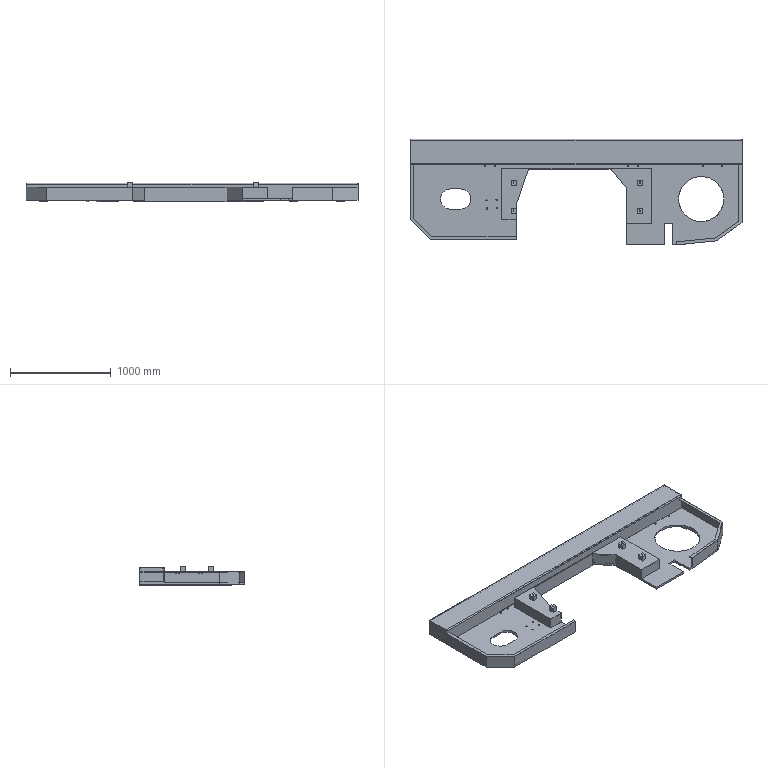Part | SolidWorks | features ICE 22, HoleWzd 5, BossThin 4, Cut 3, Rib 2, Extrusion 1, Fillet 1, WeldmentFeature 1 | 5 solids | 351 faces | box 3295 x 1050 x 195 mm | volume 87655844 mm3 | plane 194 | cylinder 157 | commonest cylinder face diameters 12 x52 9 x44 4.2 x16 6.8 x16 30 x16 20 x8